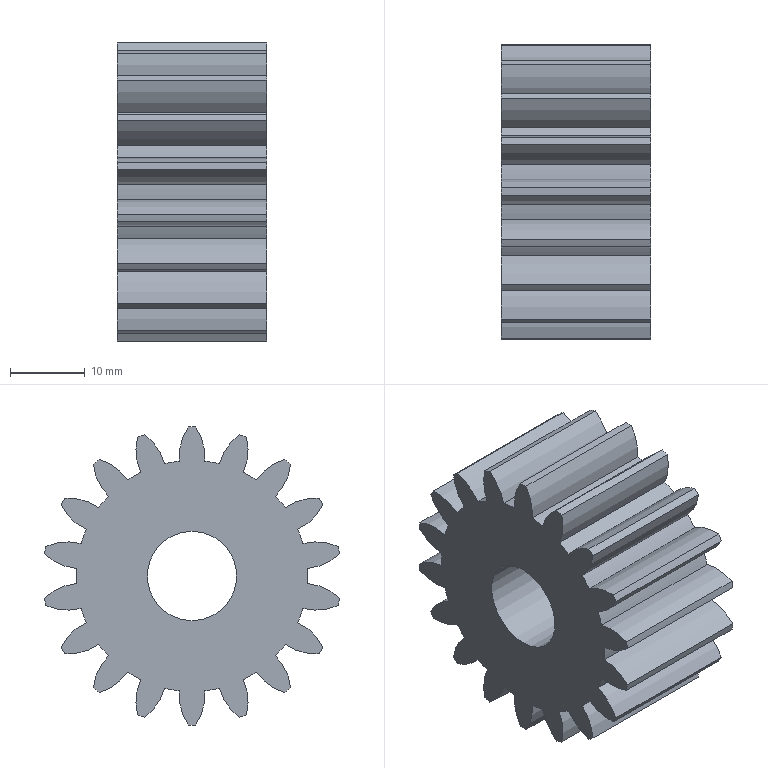Part | STEP file | spur gear_gb_GB - Spur gear 2M 18T 20PA 20FW ---S18A75H50L12.0N | 1 solid | 75 faces | box 20 x 39.557 x 40 mm | volume 17312 mm3 | cylinder 73 | plane 2 | commonest cylinder face diameters 14.4 x36 30.998 x18 40 x18 12 x1